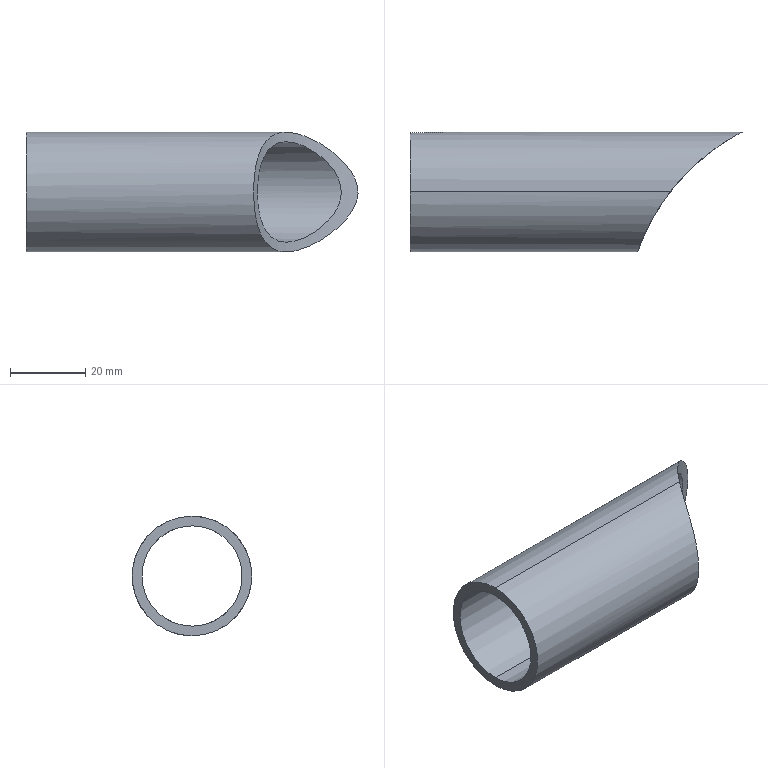Part | SolidWorks | features Extrusion 1 | 1 solid | 6 faces | box 88.118 x 31.75 x 31.75 mm | volume 16665 mm3 | cylinder 5 | plane 1 | commonest cylinder face diameters 26.645 x2 31.75 x2 114.3 x1
STEP:
#1=CARTESIAN_POINT('',(-45.237,34.925,177.178));
#2=VERTEX_POINT('',#1);
#3=CARTESIAN_POINT('',(-45.237,34.925,203.822));
#4=VERTEX_POINT('',#3);
#5=CARTESIAN_POINT('',(-45.237,34.925,177.178));
#6=CARTESIAN_POINT('',(-45.814,34.177,177.178));
#7=CARTESIAN_POINT('',(-46.369,33.42,177.24));
#8=CARTESIAN_POINT('',(-47.169,32.272,177.439));
#9=CARTESIAN_POINT('',(-47.429,31.887,177.523));
#10=CARTESIAN_POINT('',(-47.94,31.114,177.728));
#11=CARTESIAN_POINT('',(-48.19,30.725,177.85));
#12=CARTESIAN_POINT('',(-48.911,29.574,178.272));
#13=CARTESIAN_POINT('',(-49.356,28.824,178.627));
#14=CARTESIAN_POINT('',(-49.974,27.729,179.28));
#15=CARTESIAN_POINT('',(-50.171,27.37,179.518));
#16=CARTESIAN_POINT('',(-50.55,26.664,180.039));
#17=CARTESIAN_POINT('',(-50.728,26.324,180.317));
#18=CARTESIAN_POINT('',(-51.229,25.343,181.203));
#19=CARTESIAN_POINT('',(-51.52,24.741,181.862));
#20=CARTESIAN_POINT('',(-51.9,23.93,182.964));
#21=CARTESIAN_POINT('',(-52.017,23.673,183.352));
#22=CARTESIAN_POINT('',(-52.228,23.204,184.151));
#23=CARTESIAN_POINT('',(-52.322,22.99,184.562));
#24=CARTESIAN_POINT('',(-52.489,22.607,185.405));
#25=CARTESIAN_POINT('',(-52.562,22.436,185.838));
#26=CARTESIAN_POINT('',(-52.688,22.14,186.727));
#27=CARTESIAN_POINT('',(-52.741,22.013,187.185));
#28=CARTESIAN_POINT('',(-52.867,21.708,188.577));
#29=CARTESIAN_POINT('',(-52.909,21.606,189.514));
#30=CARTESIAN_POINT('',(-52.91,21.601,190.933));
#31=CARTESIAN_POINT('',(-52.901,21.625,191.411));
#32=CARTESIAN_POINT('',(-52.86,21.724,192.359));
#33=CARTESIAN_POINT('',(-52.829,21.799,192.826));
#34=CARTESIAN_POINT('',(-52.748,21.996,193.745));
#35=CARTESIAN_POINT('',(-52.697,22.118,194.199));
#36=CARTESIAN_POINT('',(-52.573,22.41,195.091));
#37=CARTESIAN_POINT('',(-52.5,22.581,195.533));
#38=CARTESIAN_POINT('',(-52.25,23.158,196.816));
#39=CARTESIAN_POINT('',(-52.043,23.622,197.611));
#40=CARTESIAN_POINT('',(-51.666,24.43,198.719));
#41=CARTESIAN_POINT('',(-51.528,24.72,199.076));
#42=CARTESIAN_POINT('',(-51.233,25.325,199.748));
#43=CARTESIAN_POINT('',(-51.076,25.641,200.065));
#44=CARTESIAN_POINT('',(-50.743,26.295,200.659));
#45=CARTESIAN_POINT('',(-50.566,26.634,200.937));
#46=CARTESIAN_POINT('',(-50.192,27.333,201.456));
#47=CARTESIAN_POINT('',(-49.993,27.695,201.698));
#48=CARTESIAN_POINT('',(-49.372,28.797,202.36));
#49=CARTESIAN_POINT('',(-48.926,29.55,202.717));
#50=CARTESIAN_POINT('',(-47.967,31.082,203.282));
#51=CARTESIAN_POINT('',(-47.451,31.865,203.49));
#52=CARTESIAN_POINT('',(-46.379,33.406,203.759));
#53=CARTESIAN_POINT('',(-45.82,34.17,203.822));
#54=CARTESIAN_POINT('',(-45.237,34.925,203.822));
#55=B_SPLINE_CURVE_WITH_KNOTS('',3,(#5,#6,#7,#8,#9,#10,#11,#12,#13,#14,#15,#16,#17,#18,#19,#20,#21,#22,#23,#24,#25,#26,#27,#28,#29,#30,#31,#32,#33,#34,#35,#36,#37,#38,#39,#40,#41,#42,#43,#44,#45,#46,#47,#48,#49,#50,#51,#52,#53,#54),.UNSPECIFIED.,.F.,.F.,(4,2,2,2,2,2,2,2,2,2,2,2,2,2,2,2,2,2,2,2,2,2,2,2,4),(0.0517,0.05452,0.05593,0.05735,0.06017,0.06159,0.063,0.06582,0.06724,0.06865,0.07006,0.07148,0.0743,0.07571,0.07713,0.07854,0.07995,0.08278,0.08419,0.0856,0.08702,0.08843,0.09126,0.09408,0.09691),.UNSPECIFIED.);
#56=EDGE_CURVE('',#2,#4,#55,.T.);
#57=ORIENTED_EDGE('',*,*,#56,.F.);
#58=CARTESIAN_POINT('',(-114.3,34.925,177.178));
#59=VERTEX_POINT('',#58);
#60=CARTESIAN_POINT('',(57.151,34.925,177.178));
#61=DIRECTION('',(-1.,0.,0.));
#62=VECTOR('',#61,1000.);
#63=LINE('',#60,#62);
#64=EDGE_CURVE('',#2,#59,#63,.T.);
#65=ORIENTED_EDGE('',*,*,#64,.T.);
#66=CARTESIAN_POINT('',(-114.3,34.925,203.822));
#67=VERTEX_POINT('',#66);
#68=CARTESIAN_POINT('',(-114.3,34.925,190.5));
#69=DIRECTION('',(-1.,0.,0.));
#70=DIRECTION('',(0.,0.,1.));
#71=AXIS2_PLACEMENT_3D('',#68,#69,#70);
#72=CIRCLE('',#71,13.322);
#73=EDGE_CURVE('',#59,#67,#72,.T.);
#74=ORIENTED_EDGE('',*,*,#73,.T.);
#75=CARTESIAN_POINT('',(57.151,34.925,203.822));
#76=DIRECTION('',(-1.,0.,0.));
#77=VECTOR('',#76,1000.);
#78=LINE('',#75,#77);
#79=EDGE_CURVE('',#4,#67,#78,.T.);
#80=ORIENTED_EDGE('',*,*,#79,.F.);
#81=EDGE_LOOP('',(#57,#65,#74,#80));
#82=FACE_OUTER_BOUND('',#81,.T.);
#83=CARTESIAN_POINT('',(57.151,34.925,190.5));
#84=DIRECTION('',(-1.,0.,0.));
#85=DIRECTION('',(0.,0.,1.));
#86=AXIS2_PLACEMENT_3D('',#83,#84,#85);
#87=CYLINDRICAL_SURFACE('',#86,13.322);
#88=ADVANCED_FACE('',(#82),#87,.F.);
#89=CARTESIAN_POINT('',(-45.237,34.925,206.375));
#90=VERTEX_POINT('',#89);
#91=CARTESIAN_POINT('',(-45.237,34.925,174.625));
#92=VERTEX_POINT('',#91);
#93=CARTESIAN_POINT('',(-45.237,34.925,206.375));
#94=CARTESIAN_POINT('',(-44.418,35.986,206.375));
#95=CARTESIAN_POINT('',(-43.573,37.003,206.27));
#96=CARTESIAN_POINT('',(-41.833,38.96,205.886));
#97=CARTESIAN_POINT('',(-40.938,39.899,205.607));
#98=CARTESIAN_POINT('',(-39.099,41.702,204.889));
#99=CARTESIAN_POINT('',(-38.172,42.551,204.455));
#100=CARTESIAN_POINT('',(-36.312,44.148,203.455));
#101=CARTESIAN_POINT('',(-35.378,44.898,202.888));
#102=CARTESIAN_POINT('',(-33.98,45.955,201.927));
#103=CARTESIAN_POINT('',(-33.513,46.296,201.588));
#104=CARTESIAN_POINT('',(-32.594,46.948,200.878));
#105=CARTESIAN_POINT('',(-32.14,47.259,200.506));
#106=CARTESIAN_POINT('',(-31.247,47.854,199.725));
#107=CARTESIAN_POINT('',(-30.809,48.137,199.315));
#108=CARTESIAN_POINT('',(-29.953,48.675,198.451));
#109=CARTESIAN_POINT('',(-29.534,48.929,197.996));
#110=CARTESIAN_POINT('',(-28.734,49.404,197.033));
#111=CARTESIAN_POINT('',(-28.355,49.621,196.529));
#112=CARTESIAN_POINT('',(-27.831,49.916,195.731));
#113=CARTESIAN_POINT('',(-27.664,50.009,195.458));
#114=CARTESIAN_POINT('',(-27.348,50.182,194.895));
#115=CARTESIAN_POINT('',(-27.198,50.263,194.604));
#116=CARTESIAN_POINT('',(-26.789,50.483,193.714));
#117=CARTESIAN_POINT('',(-26.568,50.6,193.098));
#118=CARTESIAN_POINT('',(-26.337,50.72,192.128));
#119=CARTESIAN_POINT('',(-26.278,50.751,191.796));
#120=CARTESIAN_POINT('',(-26.2,50.791,191.134));
#121=CARTESIAN_POINT('',(-26.162,50.81,190.472));
#122=CARTESIAN_POINT('',(-26.204,50.788,189.811));
#123=CARTESIAN_POINT('',(-26.286,50.746,189.149));
#124=CARTESIAN_POINT('',(-26.348,50.714,188.817));
#125=CARTESIAN_POINT('',(-26.585,50.591,187.849));
#126=CARTESIAN_POINT('',(-26.811,50.472,187.23));
#127=CARTESIAN_POINT('',(-27.365,50.173,186.041));
#128=CARTESIAN_POINT('',(-27.686,49.998,185.485));
#129=CARTESIAN_POINT('',(-28.386,49.604,184.428));
#130=CARTESIAN_POINT('',(-28.765,49.385,183.927));
#131=CARTESIAN_POINT('',(-29.567,48.909,182.968));
#132=CARTESIAN_POINT('',(-29.986,48.654,182.513));
#133=CARTESIAN_POINT('',(-30.841,48.116,181.654));
#134=CARTESIAN_POINT('',(-31.279,47.833,181.246));
#135=CARTESIAN_POINT('',(-32.614,46.943,180.081));
#136=CARTESIAN_POINT('',(-33.531,46.294,179.379));
#137=CARTESIAN_POINT('',(-34.931,45.236,178.42));
#138=CARTESIAN_POINT('',(-35.4,44.87,178.117));
#139=CARTESIAN_POINT('',(-36.333,44.118,177.549));
#140=CARTESIAN_POINT('',(-36.799,43.73,177.282));
#141=CARTESIAN_POINT('',(-38.192,42.532,176.534));
#142=CARTESIAN_POINT('',(-39.115,41.686,176.104));
#143=CARTESIAN_POINT('',(-40.487,40.34,175.569));
#144=CARTESIAN_POINT('',(-40.943,39.877,175.409));
#145=CARTESIAN_POINT('',(-41.84,38.935,175.132));
#146=CARTESIAN_POINT('',(-42.281,38.455,175.015));
#147=CARTESIAN_POINT('',(-43.585,36.989,174.728));
#148=CARTESIAN_POINT('',(-44.425,35.976,174.625));
#149=CARTESIAN_POINT('',(-45.237,34.925,174.625));
#150=B_SPLINE_CURVE_WITH_KNOTS('',3,(#93,#94,#95,#96,#97,#98,#99,#100,#101,#102,#103,#104,#105,#106,#107,#108,#109,#110,#111,#112,#113,#114,#115,#116,#117,#118,#119,#120,#121,#122,#123,#124,#125,#126,#127,#128,#129,#130,#131,#132,#133,#134,#135,#136,#137,#138,#139,#140,#141,#142,#143,#144,#145,#146,#147,#148,#149),.UNSPECIFIED.,.F.,.F.,(4,2,2,2,2,2,2,2,2,2,2,2,2,2,1,2,2,2,2,2,2,2,2,2,2,2,2,2,4),(0.,0.003969,0.007939,0.01191,0.01588,0.01786,0.01985,0.02183,0.02382,0.0258,0.02679,0.02779,0.02977,0.03076,0.03175,0.03275,0.03374,0.03572,0.03771,0.03969,0.04168,0.04366,0.04763,0.04962,0.0516,0.05557,0.05756,0.05954,0.06351),.UNSPECIFIED.);
#151=EDGE_CURVE('',#90,#92,#150,.T.);
#152=ORIENTED_EDGE('',*,*,#151,.T.);
#153=CARTESIAN_POINT('',(-114.3,34.925,174.625));
#154=VERTEX_POINT('',#153);
#155=CARTESIAN_POINT('',(57.151,34.925,174.625));
#156=DIRECTION('',(-1.,0.,0.));
#157=VECTOR('',#156,1000.);
#158=LINE('',#155,#157);
#159=EDGE_CURVE('',#92,#154,#158,.T.);
#160=ORIENTED_EDGE('',*,*,#159,.T.);
#161=CARTESIAN_POINT('',(-114.3,34.925,206.375));
#162=VERTEX_POINT('',#161);
#163=CARTESIAN_POINT('',(-114.3,34.925,190.5));
#164=DIRECTION('',(-1.,0.,0.));
#165=DIRECTION('',(0.,0.,1.));
#166=AXIS2_PLACEMENT_3D('',#163,#164,#165);
#167=CIRCLE('',#166,15.875);
#168=EDGE_CURVE('',#162,#154,#167,.T.);
#169=ORIENTED_EDGE('',*,*,#168,.F.);
#170=CARTESIAN_POINT('',(57.151,34.925,206.375));
#171=DIRECTION('',(-1.,0.,0.));
#172=VECTOR('',#171,1000.);
#173=LINE('',#170,#172);
#174=EDGE_CURVE('',#90,#162,#173,.T.);
#175=ORIENTED_EDGE('',*,*,#174,.F.);
#176=EDGE_LOOP('',(#152,#160,#169,#175));
#177=FACE_OUTER_BOUND('',#176,.T.);
#178=CARTESIAN_POINT('',(57.151,34.925,190.5));
#179=DIRECTION('',(-1.,0.,0.));
#180=DIRECTION('',(0.,0.,1.));
#181=AXIS2_PLACEMENT_3D('',#178,#179,#180);
#182=CYLINDRICAL_SURFACE('',#181,15.875);
#183=ADVANCED_FACE('',(#177),#182,.T.);
#184=ORIENTED_EDGE('',*,*,#159,.F.);
#185=CARTESIAN_POINT('',(-45.237,34.925,174.625));
#186=CARTESIAN_POINT('',(-45.579,34.482,174.625));
#187=CARTESIAN_POINT('',(-45.917,34.03,174.644));
#188=CARTESIAN_POINT('',(-46.577,33.122,174.721));
#189=CARTESIAN_POINT('',(-46.897,32.666,174.78));
#190=CARTESIAN_POINT('',(-47.832,31.297,175.017));
#191=CARTESIAN_POINT('',(-48.418,30.38,175.258));
#192=CARTESIAN_POINT('',(-49.245,29.005,175.762));
#193=CARTESIAN_POINT('',(-49.514,28.544,175.955));
#194=CARTESIAN_POINT('',(-50.024,27.64,176.386));
#195=CARTESIAN_POINT('',(-50.266,27.197,176.624));
#196=CARTESIAN_POINT('',(-50.957,25.894,177.405));
#197=CARTESIAN_POINT('',(-51.369,25.063,178.015));
#198=CARTESIAN_POINT('',(-51.921,23.885,179.08));
#199=CARTESIAN_POINT('',(-52.095,23.502,179.463));
#200=CARTESIAN_POINT('',(-52.415,22.78,180.263));
#201=CARTESIAN_POINT('',(-52.562,22.439,180.681));
#202=CARTESIAN_POINT('',(-52.964,21.48,181.99));
#203=CARTESIAN_POINT('',(-53.184,20.923,182.935));
#204=CARTESIAN_POINT('',(-53.538,20.001,184.973));
#205=CARTESIAN_POINT('',(-53.665,19.652,186.028));
#206=CARTESIAN_POINT('',(-53.794,19.296,187.662));
#207=CARTESIAN_POINT('',(-53.826,19.205,188.215));
#208=CARTESIAN_POINT('',(-53.87,19.082,189.34));
#209=CARTESIAN_POINT('',(-53.881,19.051,189.902));
#210=CARTESIAN_POINT('',(-53.882,19.047,191.581));
#211=CARTESIAN_POINT('',(-53.842,19.162,192.693));
#212=CARTESIAN_POINT('',(-53.673,19.631,194.902));
#213=CARTESIAN_POINT('',(-53.547,19.978,195.961));
#214=CARTESIAN_POINT('',(-53.288,20.654,197.475));
#215=CARTESIAN_POINT('',(-53.19,20.905,197.968));
#216=CARTESIAN_POINT('',(-52.968,21.461,198.929));
#217=CARTESIAN_POINT('',(-52.846,21.761,199.39));
#218=CARTESIAN_POINT('',(-52.444,22.72,200.709));
#219=CARTESIAN_POINT('',(-52.13,23.437,201.509));
#220=CARTESIAN_POINT('',(-51.391,25.018,202.95));
#221=CARTESIAN_POINT('',(-50.976,25.857,203.57));
#222=CARTESIAN_POINT('',(-50.283,27.166,204.359));
#223=CARTESIAN_POINT('',(-50.04,27.612,204.599));
#224=CARTESIAN_POINT('',(-49.528,28.52,205.034));
#225=CARTESIAN_POINT('',(-49.261,28.979,205.228));
#226=CARTESIAN_POINT('',(-48.434,30.355,205.734));
#227=CARTESIAN_POINT('',(-47.846,31.275,205.978));
#228=CARTESIAN_POINT('',(-46.905,32.654,206.219));
#229=CARTESIAN_POINT('',(-46.581,33.115,206.278));
#230=CARTESIAN_POINT('',(-45.92,34.026,206.356));
#231=CARTESIAN_POINT('',(-45.582,34.478,206.375));
#232=CARTESIAN_POINT('',(-45.237,34.925,206.375));
#233=B_SPLINE_CURVE_WITH_KNOTS('',3,(#185,#186,#187,#188,#189,#190,#191,#192,#193,#194,#195,#196,#197,#198,#199,#200,#201,#202,#203,#204,#205,#206,#207,#208,#209,#210,#211,#212,#213,#214,#215,#216,#217,#218,#219,#220,#221,#222,#223,#224,#225,#226,#227,#228,#229,#230,#231,#232),.UNSPECIFIED.,.F.,.F.,(4,2,2,2,2,2,2,2,2,2,2,2,2,2,2,2,2,2,2,2,2,2,2,4),(0.06351,0.06518,0.06685,0.0702,0.07187,0.07355,0.07689,0.07856,0.08024,0.08358,0.08693,0.0886,0.09027,0.09362,0.09696,0.09864,0.1003,0.1037,0.107,0.1087,0.1103,0.1137,0.1154,0.117),.UNSPECIFIED.);
#234=EDGE_CURVE('',#92,#90,#233,.T.);
#235=ORIENTED_EDGE('',*,*,#234,.T.);
#236=ORIENTED_EDGE('',*,*,#174,.T.);
#237=CARTESIAN_POINT('',(-114.3,34.925,190.5));
#238=DIRECTION('',(-1.,0.,0.));
#239=DIRECTION('',(0.,0.,1.));
#240=AXIS2_PLACEMENT_3D('',#237,#238,#239);
#241=CIRCLE('',#240,15.875);
#242=EDGE_CURVE('',#154,#162,#241,.T.);
#243=ORIENTED_EDGE('',*,*,#242,.F.);
#244=EDGE_LOOP('',(#184,#235,#236,#243));
#245=FACE_OUTER_BOUND('',#244,.T.);
#246=CARTESIAN_POINT('',(57.151,34.925,190.5));
#247=DIRECTION('',(-1.,0.,0.));
#248=DIRECTION('',(0.,0.,1.));
#249=AXIS2_PLACEMENT_3D('',#246,#247,#248);
#250=CYLINDRICAL_SURFACE('',#249,15.875);
#251=ADVANCED_FACE('',(#245),#250,.T.);
#252=CARTESIAN_POINT('',(-114.3,34.925,190.5));
#253=DIRECTION('',(-1.,0.,0.));
#254=DIRECTION('',(0.,0.,1.));
#255=AXIS2_PLACEMENT_3D('',#252,#253,#254);
#256=CIRCLE('',#255,13.322);
#257=EDGE_CURVE('',#67,#59,#256,.T.);
#258=ORIENTED_EDGE('',*,*,#257,.F.);
#259=ORIENTED_EDGE('',*,*,#73,.F.);
#260=EDGE_LOOP('',(#258,#259));
#261=FACE_BOUND('',#260,.T.);
#262=ORIENTED_EDGE('',*,*,#168,.T.);
#263=ORIENTED_EDGE('',*,*,#242,.T.);
#264=EDGE_LOOP('',(#262,#263));
#265=FACE_OUTER_BOUND('',#264,.T.);
#266=CARTESIAN_POINT('',(-114.3,34.925,190.5));
#267=DIRECTION('',(-1.,0.,0.));
#268=DIRECTION('',(0.,0.,1.));
#269=AXIS2_PLACEMENT_3D('',#266,#267,#268);
#270=PLANE('',#269);
#271=ADVANCED_FACE('',(#261,#265),#270,.T.);
#272=ORIENTED_EDGE('',*,*,#64,.F.);
#273=CARTESIAN_POINT('',(-45.237,34.925,203.822));
#274=CARTESIAN_POINT('',(-44.57,35.788,203.822));
#275=CARTESIAN_POINT('',(-43.888,36.621,203.739));
#276=CARTESIAN_POINT('',(-42.492,38.232,203.431));
#277=CARTESIAN_POINT('',(-41.778,39.01,203.206));
#278=CARTESIAN_POINT('',(-40.685,40.138,202.767));
#279=CARTESIAN_POINT('',(-40.319,40.506,202.603));
#280=CARTESIAN_POINT('',(-39.589,41.22,202.248));
#281=CARTESIAN_POINT('',(-39.224,41.567,202.055));
#282=CARTESIAN_POINT('',(-38.131,42.581,201.432));
#283=CARTESIAN_POINT('',(-37.405,43.219,200.957));
#284=CARTESIAN_POINT('',(-36.327,44.121,200.147));
#285=CARTESIAN_POINT('',(-35.968,44.414,199.86));
#286=CARTESIAN_POINT('',(-35.262,44.977,199.253));
#287=CARTESIAN_POINT('',(-34.916,45.246,198.935));
#288=CARTESIAN_POINT('',(-34.241,45.759,198.265));
#289=CARTESIAN_POINT('',(-33.911,46.003,197.913));
#290=CARTESIAN_POINT('',(-33.275,46.466,197.17));
#291=CARTESIAN_POINT('',(-32.966,46.685,196.777));
#292=CARTESIAN_POINT('',(-32.384,47.091,195.949));
#293=CARTESIAN_POINT('',(-32.113,47.276,195.518));
#294=CARTESIAN_POINT('',(-31.621,47.606,194.612));
#295=CARTESIAN_POINT('',(-31.4,47.752,194.136));
#296=CARTESIAN_POINT('',(-31.028,47.994,193.135));
#297=CARTESIAN_POINT('',(-30.882,48.088,192.622));
#298=CARTESIAN_POINT('',(-30.732,48.184,191.828));
#299=CARTESIAN_POINT('',(-30.694,48.208,191.56));
#300=CARTESIAN_POINT('',(-30.643,48.24,191.015));
#301=CARTESIAN_POINT('',(-30.631,48.248,190.741));
#302=CARTESIAN_POINT('',(-30.634,48.246,189.928));
#303=CARTESIAN_POINT('',(-30.688,48.212,189.392));
#304=CARTESIAN_POINT('',(-30.843,48.113,188.594));
#305=CARTESIAN_POINT('',(-30.907,48.072,188.329));
#306=CARTESIAN_POINT('',(-31.055,47.976,187.815));
#307=CARTESIAN_POINT('',(-31.139,47.922,187.563));
#308=CARTESIAN_POINT('',(-31.418,47.74,186.823));
#309=CARTESIAN_POINT('',(-31.639,47.594,186.351));
#310=CARTESIAN_POINT('',(-32.139,47.258,185.438));
#311=CARTESIAN_POINT('',(-32.412,47.071,185.008));
#312=CARTESIAN_POINT('',(-32.991,46.667,184.191));
#313=CARTESIAN_POINT('',(-33.297,46.45,183.803));
#314=CARTESIAN_POINT('',(-33.933,45.987,183.063));
#315=CARTESIAN_POINT('',(-34.265,45.741,182.71));
#316=CARTESIAN_POINT('',(-35.286,44.964,181.701));
#317=CARTESIAN_POINT('',(-35.988,44.405,181.106));
#318=CARTESIAN_POINT('',(-37.416,43.209,180.036));
#319=CARTESIAN_POINT('',(-38.141,42.572,179.562));
#320=CARTESIAN_POINT('',(-39.239,41.553,178.937));
#321=CARTESIAN_POINT('',(-39.608,41.202,178.742));
#322=CARTESIAN_POINT('',(-40.338,40.487,178.388));
#323=CARTESIAN_POINT('',(-40.701,40.123,178.227));
#324=CARTESIAN_POINT('',(-41.781,39.007,177.793));
#325=CARTESIAN_POINT('',(-42.49,38.234,177.569));
#326=CARTESIAN_POINT('',(-43.536,37.027,177.338));
#327=CARTESIAN_POINT('',(-43.882,36.617,177.279));
#328=CARTESIAN_POINT('',(-44.568,35.779,177.198));
#329=CARTESIAN_POINT('',(-44.907,35.353,177.178));
#330=CARTESIAN_POINT('',(-45.237,34.925,177.178));
#331=B_SPLINE_CURVE_WITH_KNOTS('',3,(#273,#274,#275,#276,#277,#278,#279,#280,#281,#282,#283,#284,#285,#286,#287,#288,#289,#290,#291,#292,#293,#294,#295,#296,#297,#298,#299,#300,#301,#302,#303,#304,#305,#306,#307,#308,#309,#310,#311,#312,#313,#314,#315,#316,#317,#318,#319,#320,#321,#322,#323,#324,#325,#326,#327,#328,#329,#330),.UNSPECIFIED.,.F.,.F.,(4,2,2,2,2,2,2,2,2,2,2,2,2,2,2,2,2,2,2,2,2,2,2,2,2,2,2,2,4),(0.,0.003231,0.006462,0.008078,0.009693,0.01292,0.01454,0.01616,0.01777,0.01939,0.021,0.02262,0.02423,0.02504,0.02585,0.02746,0.02827,0.02908,0.03069,0.03231,0.03393,0.03554,0.03877,0.042,0.04362,0.04523,0.04847,0.05008,0.0517),.UNSPECIFIED.);
#332=EDGE_CURVE('',#4,#2,#331,.T.);
#333=ORIENTED_EDGE('',*,*,#332,.F.);
#334=ORIENTED_EDGE('',*,*,#79,.T.);
#335=ORIENTED_EDGE('',*,*,#257,.T.);
#336=EDGE_LOOP('',(#272,#333,#334,#335));
#337=FACE_OUTER_BOUND('',#336,.T.);
#338=CARTESIAN_POINT('',(57.151,34.925,190.5));
#339=DIRECTION('',(-1.,0.,0.));
#340=DIRECTION('',(0.,0.,1.));
#341=AXIS2_PLACEMENT_3D('',#338,#339,#340);
#342=CYLINDRICAL_SURFACE('',#341,13.322);
#343=ADVANCED_FACE('',(#337),#342,.F.);
#344=ORIENTED_EDGE('',*,*,#151,.F.);
#345=ORIENTED_EDGE('',*,*,#234,.F.);
#346=EDGE_LOOP('',(#344,#345));
#347=FACE_OUTER_BOUND('',#346,.T.);
#348=ORIENTED_EDGE('',*,*,#332,.T.);
#349=ORIENTED_EDGE('',*,*,#56,.T.);
#350=EDGE_LOOP('',(#348,#349));
#351=FACE_BOUND('',#350,.T.);
#352=CARTESIAN_POINT('',(0.,0.,222.25));
#353=DIRECTION('',(0.,0.,-1.));
#354=DIRECTION('',(-1.,0.,0.));
#355=AXIS2_PLACEMENT_3D('',#352,#353,#354);
#356=CYLINDRICAL_SURFACE('',#355,57.15);
#357=ADVANCED_FACE('',(#347,#351),#356,.F.);
#358=CLOSED_SHELL('',(#88,#183,#251,#271,#343,#357));
#359=MANIFOLD_SOLID_BREP('',#358);
#360=CARTESIAN_POINT('',(0.,0.,0.));
#361=DIRECTION('',(0.,0.,1.));
#362=DIRECTION('',(1.,0.,0.));
#363=AXIS2_PLACEMENT_3D('',#360,#361,#362);
#364=(LENGTH_UNIT()NAMED_UNIT(*)SI_UNIT(.MILLI.,.METRE.));
#365=UNCERTAINTY_MEASURE_WITH_UNIT(LENGTH_MEASURE(0.00001),#364,'','');
#366=(NAMED_UNIT(*)PLANE_ANGLE_UNIT()SI_UNIT($,.RADIAN.));
#367=(NAMED_UNIT(*)SI_UNIT($,.STERADIAN.)SOLID_ANGLE_UNIT());
#368=(GEOMETRIC_REPRESENTATION_CONTEXT(3)GLOBAL_UNCERTAINTY_ASSIGNED_CONTEXT((#365))GLOBAL_UNIT_ASSIGNED_CONTEXT((#364,#366,#367))REPRESENTATION_CONTEXT('',''));
#369=ADVANCED_BREP_SHAPE_REPRESENTATION('',(#359,#363),#368);